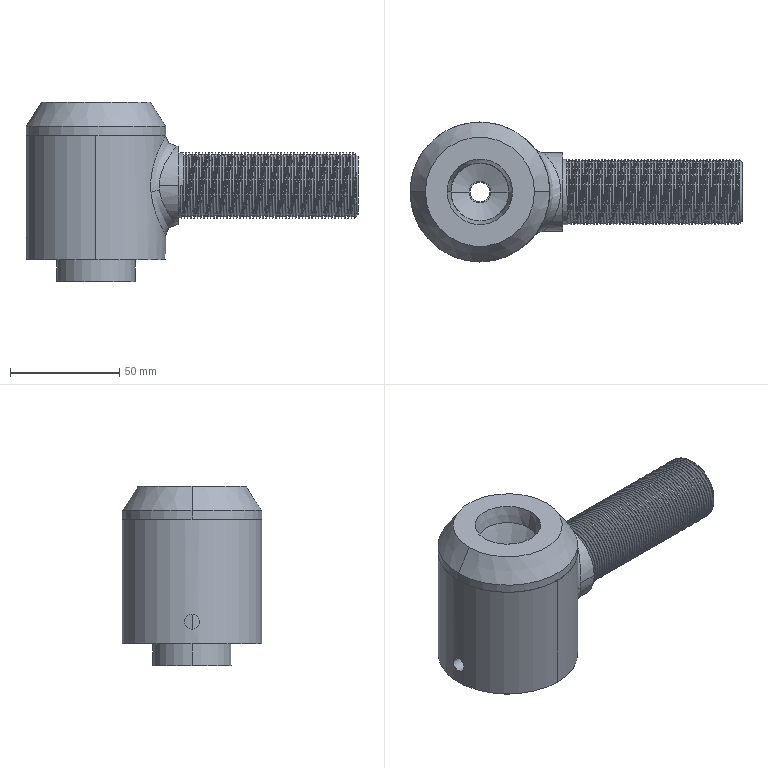Part | SolidWorks | 4 solids | 187 faces | box 152 x 64 x 82 mm | volume 214703 mm3 | cylinder 137 | cone 22 | plane 21 | spline 4 | sphere 3 | commonest cylinder face diameters 30 x106 50 x5 4 x4 36 x4 52 x4 64 x4